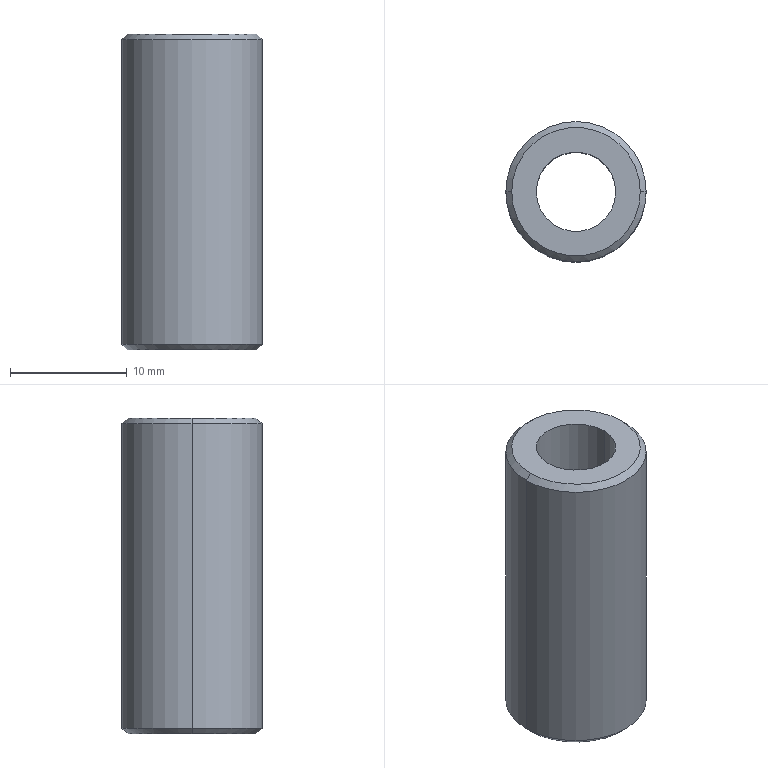Part | STEP file | Screw sleeve QY-1-33 | 1 solid | 10 faces | box 12 x 12 x 27 mm | volume 2064 mm3 | cone 4 | cylinder 4 | plane 2 | commonest cylinder face diameters 6.8 x2 12 x2
STEP:
#1=CARTESIAN_POINT('',(0.,0.,0.));
#2=DIRECTION('',(0.,0.,1.));
#3=DIRECTION('',(1.,0.,0.));
#4=AXIS2_PLACEMENT_3D('',#1,#2,#3);
#5=CARTESIAN_POINT('',(-5.5,0.,0.));
#6=VERTEX_POINT('',#5);
#7=CARTESIAN_POINT('',(5.5,0.,0.));
#8=VERTEX_POINT('',#7);
#9=CARTESIAN_POINT('',(0.,0.,0.));
#10=DIRECTION('',(0.,0.,-1.));
#11=DIRECTION('',(1.,0.,0.));
#12=AXIS2_PLACEMENT_3D('',#9,#10,#11);
#13=CIRCLE('',#12,5.5);
#14=CARTESIAN_POINT('',(0.,0.,0.5));
#15=DIRECTION('',(0.,0.,1.));
#16=DIRECTION('',(1.,0.,0.));
#17=AXIS2_PLACEMENT_3D('',#14,#15,#16);
#18=CONICAL_SURFACE('',#17,6.,0.7854);
#19=CARTESIAN_POINT('',(6.283,-0.5));
#20=DIRECTION('',(-1.,0.));
#21=VECTOR('',#20,1.);
#22=LINE('',#19,#21);
#23=(GEOMETRIC_REPRESENTATION_CONTEXT(2)PARAMETRIC_REPRESENTATION_CONTEXT()REPRESENTATION_CONTEXT('',''));
#24=DEFINITIONAL_REPRESENTATION('',(#22),#23);
#25=PCURVE('',#18,#24);
#26=CARTESIAN_POINT('',(0.,0.,0.));
#27=DIRECTION('',(0.,0.,1.));
#28=DIRECTION('',(1.,0.,0.));
#29=AXIS2_PLACEMENT_3D('',#26,#27,#28);
#30=PLANE('',#29);
#31=CARTESIAN_POINT('',(5.5,0.));
#32=CARTESIAN_POINT('',(5.5,-9.526));
#33=CARTESIAN_POINT('',(-2.75,-4.763));
#34=CARTESIAN_POINT('',(-11.,0.));
#35=CARTESIAN_POINT('',(-2.75,4.763));
#36=CARTESIAN_POINT('',(5.5,9.526));
#37=CARTESIAN_POINT('',(5.5,0.));
#38=(BOUNDED_CURVE()B_SPLINE_CURVE(2,(#31,#32,#33,#34,#35,#36,#37),.UNSPECIFIED.,.T.,.F.)B_SPLINE_CURVE_WITH_KNOTS((1,2,2,2,2,1),(-2.094,0.,2.094,4.189,6.283,8.378),.UNSPECIFIED.)CURVE()GEOMETRIC_REPRESENTATION_ITEM()RATIONAL_B_SPLINE_CURVE((1.,0.5,1.,0.5,1.,0.5,1.))REPRESENTATION_ITEM(''));
#39=(GEOMETRIC_REPRESENTATION_CONTEXT(2)PARAMETRIC_REPRESENTATION_CONTEXT()REPRESENTATION_CONTEXT('',''));
#40=DEFINITIONAL_REPRESENTATION('',(#38),#39);
#41=PCURVE('',#30,#40);
#42=SURFACE_CURVE('',#13,(#25,#41),.PCURVE_S1.);
#43=EDGE_CURVE('',#6,#8,#42,.T.);
#44=ORIENTED_EDGE('',*,*,#43,.F.);
#45=CARTESIAN_POINT('',(-6.,0.,0.5));
#46=VERTEX_POINT('',#45);
#47=CARTESIAN_POINT('',(-6.,0.,0.5));
#48=DIRECTION('',(-0.7071,0.,0.7071));
#49=VECTOR('',#48,1.);
#50=LINE('',#47,#49);
#51=CARTESIAN_POINT('',(3.142,0.));
#52=DIRECTION('',(0.,1.));
#53=VECTOR('',#52,1.);
#54=LINE('',#51,#53);
#55=(GEOMETRIC_REPRESENTATION_CONTEXT(2)PARAMETRIC_REPRESENTATION_CONTEXT()REPRESENTATION_CONTEXT('',''));
#56=DEFINITIONAL_REPRESENTATION('',(#54),#55);
#57=PCURVE('',#18,#56);
#58=CARTESIAN_POINT('',(0.,0.,0.5));
#59=DIRECTION('',(0.,0.,1.));
#60=DIRECTION('',(1.,0.,0.));
#61=AXIS2_PLACEMENT_3D('',#58,#59,#60);
#62=CONICAL_SURFACE('',#61,6.,0.7854);
#63=CARTESIAN_POINT('',(3.142,0.));
#64=DIRECTION('',(0.,1.));
#65=VECTOR('',#64,1.);
#66=LINE('',#63,#65);
#67=(GEOMETRIC_REPRESENTATION_CONTEXT(2)PARAMETRIC_REPRESENTATION_CONTEXT()REPRESENTATION_CONTEXT('',''));
#68=DEFINITIONAL_REPRESENTATION('',(#66),#67);
#69=PCURVE('',#62,#68);
#70=SURFACE_CURVE('',#50,(#57,#69),.PCURVE_S1.);
#71=EDGE_CURVE('',#6,#46,#70,.T.);
#72=ORIENTED_EDGE('',*,*,#71,.T.);
#73=CARTESIAN_POINT('',(6.,0.,0.5));
#74=VERTEX_POINT('',#73);
#75=CARTESIAN_POINT('',(0.,0.,0.5));
#76=DIRECTION('',(0.,0.,1.));
#77=DIRECTION('',(1.,0.,0.));
#78=AXIS2_PLACEMENT_3D('',#75,#76,#77);
#79=CIRCLE('',#78,6.);
#80=CARTESIAN_POINT('',(0.,0.));
#81=DIRECTION('',(1.,0.));
#82=VECTOR('',#81,1.);
#83=LINE('',#80,#82);
#84=(GEOMETRIC_REPRESENTATION_CONTEXT(2)PARAMETRIC_REPRESENTATION_CONTEXT()REPRESENTATION_CONTEXT('',''));
#85=DEFINITIONAL_REPRESENTATION('',(#83),#84);
#86=PCURVE('',#18,#85);
#87=CARTESIAN_POINT('',(0.,0.,27.));
#88=DIRECTION('',(0.,0.,-1.));
#89=DIRECTION('',(-1.,0.,0.));
#90=AXIS2_PLACEMENT_3D('',#87,#88,#89);
#91=CYLINDRICAL_SURFACE('',#90,6.);
#92=CARTESIAN_POINT('',(3.142,26.5));
#93=DIRECTION('',(-1.,0.));
#94=VECTOR('',#93,1.);
#95=LINE('',#92,#94);
#96=(GEOMETRIC_REPRESENTATION_CONTEXT(2)PARAMETRIC_REPRESENTATION_CONTEXT()REPRESENTATION_CONTEXT('',''));
#97=DEFINITIONAL_REPRESENTATION('',(#95),#96);
#98=PCURVE('',#91,#97);
#99=SURFACE_CURVE('',#79,(#86,#98),.PCURVE_S1.);
#100=EDGE_CURVE('',#74,#46,#99,.T.);
#101=ORIENTED_EDGE('',*,*,#100,.F.);
#102=CARTESIAN_POINT('',(6.,0.,0.5));
#103=DIRECTION('',(0.7071,0.,0.7071));
#104=VECTOR('',#103,1.);
#105=LINE('',#102,#104);
#106=CARTESIAN_POINT('',(0.,0.));
#107=DIRECTION('',(0.,1.));
#108=VECTOR('',#107,1.);
#109=LINE('',#106,#108);
#110=(GEOMETRIC_REPRESENTATION_CONTEXT(2)PARAMETRIC_REPRESENTATION_CONTEXT()REPRESENTATION_CONTEXT('',''));
#111=DEFINITIONAL_REPRESENTATION('',(#109),#110);
#112=PCURVE('',#18,#111);
#113=CARTESIAN_POINT('',(6.283,0.));
#114=DIRECTION('',(0.,1.));
#115=VECTOR('',#114,1.);
#116=LINE('',#113,#115);
#117=(GEOMETRIC_REPRESENTATION_CONTEXT(2)PARAMETRIC_REPRESENTATION_CONTEXT()REPRESENTATION_CONTEXT('',''));
#118=DEFINITIONAL_REPRESENTATION('',(#116),#117);
#119=PCURVE('',#62,#118);
#120=SURFACE_CURVE('',#105,(#112,#119),.PCURVE_S1.);
#121=EDGE_CURVE('',#8,#74,#120,.T.);
#122=ORIENTED_EDGE('',*,*,#121,.F.);
#123=EDGE_LOOP('',(#44,#72,#101,#122));
#124=FACE_BOUND('',#123,.T.);
#125=ADVANCED_FACE('',(#124),#18,.T.);
#126=CARTESIAN_POINT('',(5.5,0.,27.));
#127=VERTEX_POINT('',#126);
#128=CARTESIAN_POINT('',(-5.5,0.,27.));
#129=VERTEX_POINT('',#128);
#130=CARTESIAN_POINT('',(0.,0.,27.));
#131=DIRECTION('',(0.,0.,1.));
#132=DIRECTION('',(1.,0.,0.));
#133=AXIS2_PLACEMENT_3D('',#130,#131,#132);
#134=CIRCLE('',#133,5.5);
#135=CARTESIAN_POINT('',(0.,0.,27.));
#136=DIRECTION('',(0.,0.,-1.));
#137=DIRECTION('',(-1.,0.,0.));
#138=AXIS2_PLACEMENT_3D('',#135,#136,#137);
#139=CONICAL_SURFACE('',#138,5.5,0.7854);
#140=CARTESIAN_POINT('',(3.142,0.));
#141=DIRECTION('',(-1.,0.));
#142=VECTOR('',#141,1.);
#143=LINE('',#140,#142);
#144=(GEOMETRIC_REPRESENTATION_CONTEXT(2)PARAMETRIC_REPRESENTATION_CONTEXT()REPRESENTATION_CONTEXT('',''));
#145=DEFINITIONAL_REPRESENTATION('',(#143),#144);
#146=PCURVE('',#139,#145);
#147=CARTESIAN_POINT('',(0.,0.,27.));
#148=DIRECTION('',(0.,0.,1.));
#149=DIRECTION('',(1.,0.,0.));
#150=AXIS2_PLACEMENT_3D('',#147,#148,#149);
#151=PLANE('',#150);
#152=CARTESIAN_POINT('',(0.,0.));
#153=DIRECTION('',(1.,0.));
#154=AXIS2_PLACEMENT_2D('',#152,#153);
#155=CIRCLE('',#154,5.5);
#156=(GEOMETRIC_REPRESENTATION_CONTEXT(2)PARAMETRIC_REPRESENTATION_CONTEXT()REPRESENTATION_CONTEXT('',''));
#157=DEFINITIONAL_REPRESENTATION('',(#155),#156);
#158=PCURVE('',#151,#157);
#159=SURFACE_CURVE('',#134,(#146,#158),.PCURVE_S1.);
#160=EDGE_CURVE('',#127,#129,#159,.T.);
#161=ORIENTED_EDGE('',*,*,#160,.F.);
#162=CARTESIAN_POINT('',(6.,0.,26.5));
#163=VERTEX_POINT('',#162);
#164=CARTESIAN_POINT('',(5.5,0.,27.));
#165=DIRECTION('',(0.7071,0.,-0.7071));
#166=VECTOR('',#165,1.);
#167=LINE('',#164,#166);
#168=CARTESIAN_POINT('',(3.142,0.));
#169=DIRECTION('',(0.,1.));
#170=VECTOR('',#169,1.);
#171=LINE('',#168,#170);
#172=(GEOMETRIC_REPRESENTATION_CONTEXT(2)PARAMETRIC_REPRESENTATION_CONTEXT()REPRESENTATION_CONTEXT('',''));
#173=DEFINITIONAL_REPRESENTATION('',(#171),#172);
#174=PCURVE('',#139,#173);
#175=CARTESIAN_POINT('',(0.,0.,27.));
#176=DIRECTION('',(0.,0.,-1.));
#177=DIRECTION('',(-1.,0.,0.));
#178=AXIS2_PLACEMENT_3D('',#175,#176,#177);
#179=CONICAL_SURFACE('',#178,5.5,0.7854);
#180=CARTESIAN_POINT('',(3.142,0.));
#181=DIRECTION('',(0.,1.));
#182=VECTOR('',#181,1.);
#183=LINE('',#180,#182);
#184=(GEOMETRIC_REPRESENTATION_CONTEXT(2)PARAMETRIC_REPRESENTATION_CONTEXT()REPRESENTATION_CONTEXT('',''));
#185=DEFINITIONAL_REPRESENTATION('',(#183),#184);
#186=PCURVE('',#179,#185);
#187=SURFACE_CURVE('',#167,(#174,#186),.PCURVE_S1.);
#188=EDGE_CURVE('',#127,#163,#187,.T.);
#189=ORIENTED_EDGE('',*,*,#188,.T.);
#190=CARTESIAN_POINT('',(-6.,0.,26.5));
#191=VERTEX_POINT('',#190);
#192=CARTESIAN_POINT('',(0.,0.,26.5));
#193=DIRECTION('',(0.,0.,-1.));
#194=DIRECTION('',(1.,0.,0.));
#195=AXIS2_PLACEMENT_3D('',#192,#193,#194);
#196=CIRCLE('',#195,6.);
#197=CARTESIAN_POINT('',(-3.142,0.5));
#198=DIRECTION('',(1.,0.));
#199=VECTOR('',#198,1.);
#200=LINE('',#197,#199);
#201=(GEOMETRIC_REPRESENTATION_CONTEXT(2)PARAMETRIC_REPRESENTATION_CONTEXT()REPRESENTATION_CONTEXT('',''));
#202=DEFINITIONAL_REPRESENTATION('',(#200),#201);
#203=PCURVE('',#139,#202);
#204=CARTESIAN_POINT('',(-3.142,0.5));
#205=DIRECTION('',(1.,0.));
#206=VECTOR('',#205,1.);
#207=LINE('',#204,#206);
#208=(GEOMETRIC_REPRESENTATION_CONTEXT(2)PARAMETRIC_REPRESENTATION_CONTEXT()REPRESENTATION_CONTEXT('',''));
#209=DEFINITIONAL_REPRESENTATION('',(#207),#208);
#210=PCURVE('',#91,#209);
#211=SURFACE_CURVE('',#196,(#203,#210),.PCURVE_S1.);
#212=EDGE_CURVE('',#191,#163,#211,.T.);
#213=ORIENTED_EDGE('',*,*,#212,.F.);
#214=CARTESIAN_POINT('',(-5.5,0.,27.));
#215=DIRECTION('',(-0.7071,0.,-0.7071));
#216=VECTOR('',#215,1.);
#217=LINE('',#214,#216);
#218=CARTESIAN_POINT('',(0.,0.));
#219=DIRECTION('',(0.,1.));
#220=VECTOR('',#219,1.);
#221=LINE('',#218,#220);
#222=(GEOMETRIC_REPRESENTATION_CONTEXT(2)PARAMETRIC_REPRESENTATION_CONTEXT()REPRESENTATION_CONTEXT('',''));
#223=DEFINITIONAL_REPRESENTATION('',(#221),#222);
#224=PCURVE('',#139,#223);
#225=CARTESIAN_POINT('',(6.283,0.));
#226=DIRECTION('',(0.,1.));
#227=VECTOR('',#226,1.);
#228=LINE('',#225,#227);
#229=(GEOMETRIC_REPRESENTATION_CONTEXT(2)PARAMETRIC_REPRESENTATION_CONTEXT()REPRESENTATION_CONTEXT('',''));
#230=DEFINITIONAL_REPRESENTATION('',(#228),#229);
#231=PCURVE('',#179,#230);
#232=SURFACE_CURVE('',#217,(#224,#231),.PCURVE_S1.);
#233=EDGE_CURVE('',#129,#191,#232,.T.);
#234=ORIENTED_EDGE('',*,*,#233,.F.);
#235=EDGE_LOOP('',(#161,#189,#213,#234));
#236=FACE_BOUND('',#235,.T.);
#237=ADVANCED_FACE('',(#236),#139,.T.);
#238=CARTESIAN_POINT('',(3.4,0.,0.));
#239=VERTEX_POINT('',#238);
#240=CARTESIAN_POINT('',(3.4,0.,27.));
#241=VERTEX_POINT('',#240);
#242=CARTESIAN_POINT('',(3.4,0.,27.));
#243=DIRECTION('',(0.,0.,1.));
#244=VECTOR('',#243,1.);
#245=LINE('',#242,#244);
#246=CARTESIAN_POINT('',(0.,0.,27.));
#247=DIRECTION('',(0.,0.,1.));
#248=DIRECTION('',(1.,0.,0.));
#249=AXIS2_PLACEMENT_3D('',#246,#247,#248);
#250=CYLINDRICAL_SURFACE('',#249,3.4);
#251=CARTESIAN_POINT('',(6.283,0.));
#252=DIRECTION('',(0.,1.));
#253=VECTOR('',#252,1.);
#254=LINE('',#251,#253);
#255=(GEOMETRIC_REPRESENTATION_CONTEXT(2)PARAMETRIC_REPRESENTATION_CONTEXT()REPRESENTATION_CONTEXT('',''));
#256=DEFINITIONAL_REPRESENTATION('',(#254),#255);
#257=PCURVE('',#250,#256);
#258=CARTESIAN_POINT('',(0.,0.,27.));
#259=DIRECTION('',(0.,0.,1.));
#260=DIRECTION('',(1.,0.,0.));
#261=AXIS2_PLACEMENT_3D('',#258,#259,#260);
#262=CYLINDRICAL_SURFACE('',#261,3.4);
#263=CARTESIAN_POINT('',(0.,0.));
#264=DIRECTION('',(0.,1.));
#265=VECTOR('',#264,1.);
#266=LINE('',#263,#265);
#267=(GEOMETRIC_REPRESENTATION_CONTEXT(2)PARAMETRIC_REPRESENTATION_CONTEXT()REPRESENTATION_CONTEXT('',''));
#268=DEFINITIONAL_REPRESENTATION('',(#266),#267);
#269=PCURVE('',#262,#268);
#270=SURFACE_CURVE('',#245,(#257,#269),.PCURVE_S1.);
#271=EDGE_CURVE('',#239,#241,#270,.T.);
#272=ORIENTED_EDGE('',*,*,#271,.T.);
#273=CARTESIAN_POINT('',(-3.4,0.,27.));
#274=VERTEX_POINT('',#273);
#275=CARTESIAN_POINT('',(0.,0.,27.));
#276=DIRECTION('',(0.,0.,1.));
#277=DIRECTION('',(1.,0.,0.));
#278=AXIS2_PLACEMENT_3D('',#275,#276,#277);
#279=CIRCLE('',#278,3.4);
#280=CARTESIAN_POINT('',(0.,0.));
#281=DIRECTION('',(1.,0.));
#282=VECTOR('',#281,1.);
#283=LINE('',#280,#282);
#284=(GEOMETRIC_REPRESENTATION_CONTEXT(2)PARAMETRIC_REPRESENTATION_CONTEXT()REPRESENTATION_CONTEXT('',''));
#285=DEFINITIONAL_REPRESENTATION('',(#283),#284);
#286=PCURVE('',#250,#285);
#287=CARTESIAN_POINT('',(0.,0.));
#288=DIRECTION('',(1.,0.));
#289=AXIS2_PLACEMENT_2D('',#287,#288);
#290=CIRCLE('',#289,3.4);
#291=(GEOMETRIC_REPRESENTATION_CONTEXT(2)PARAMETRIC_REPRESENTATION_CONTEXT()REPRESENTATION_CONTEXT('',''));
#292=DEFINITIONAL_REPRESENTATION('',(#290),#291);
#293=PCURVE('',#151,#292);
#294=SURFACE_CURVE('',#279,(#286,#293),.PCURVE_S1.);
#295=EDGE_CURVE('',#274,#241,#294,.T.);
#296=ORIENTED_EDGE('',*,*,#295,.F.);
#297=CARTESIAN_POINT('',(-3.4,0.,0.));
#298=VERTEX_POINT('',#297);
#299=CARTESIAN_POINT('',(-3.4,0.,27.));
#300=DIRECTION('',(0.,0.,1.));
#301=VECTOR('',#300,1.);
#302=LINE('',#299,#301);
#303=CARTESIAN_POINT('',(3.142,0.));
#304=DIRECTION('',(0.,1.));
#305=VECTOR('',#304,1.);
#306=LINE('',#303,#305);
#307=(GEOMETRIC_REPRESENTATION_CONTEXT(2)PARAMETRIC_REPRESENTATION_CONTEXT()REPRESENTATION_CONTEXT('',''));
#308=DEFINITIONAL_REPRESENTATION('',(#306),#307);
#309=PCURVE('',#250,#308);
#310=CARTESIAN_POINT('',(3.142,0.));
#311=DIRECTION('',(0.,1.));
#312=VECTOR('',#311,1.);
#313=LINE('',#310,#312);
#314=(GEOMETRIC_REPRESENTATION_CONTEXT(2)PARAMETRIC_REPRESENTATION_CONTEXT()REPRESENTATION_CONTEXT('',''));
#315=DEFINITIONAL_REPRESENTATION('',(#313),#314);
#316=PCURVE('',#262,#315);
#317=SURFACE_CURVE('',#302,(#309,#316),.PCURVE_S1.);
#318=EDGE_CURVE('',#298,#274,#317,.T.);
#319=ORIENTED_EDGE('',*,*,#318,.F.);
#320=CARTESIAN_POINT('',(0.,0.,0.));
#321=DIRECTION('',(0.,0.,1.));
#322=DIRECTION('',(1.,0.,0.));
#323=AXIS2_PLACEMENT_3D('',#320,#321,#322);
#324=CIRCLE('',#323,3.4);
#325=CARTESIAN_POINT('',(0.,-27.));
#326=DIRECTION('',(1.,0.));
#327=VECTOR('',#326,1.);
#328=LINE('',#325,#327);
#329=(GEOMETRIC_REPRESENTATION_CONTEXT(2)PARAMETRIC_REPRESENTATION_CONTEXT()REPRESENTATION_CONTEXT('',''));
#330=DEFINITIONAL_REPRESENTATION('',(#328),#329);
#331=PCURVE('',#250,#330);
#332=CARTESIAN_POINT('',(0.,0.));
#333=DIRECTION('',(1.,0.));
#334=AXIS2_PLACEMENT_2D('',#332,#333);
#335=CIRCLE('',#334,3.4);
#336=(GEOMETRIC_REPRESENTATION_CONTEXT(2)PARAMETRIC_REPRESENTATION_CONTEXT()REPRESENTATION_CONTEXT('',''));
#337=DEFINITIONAL_REPRESENTATION('',(#335),#336);
#338=PCURVE('',#30,#337);
#339=SURFACE_CURVE('',#324,(#331,#338),.PCURVE_S1.);
#340=EDGE_CURVE('',#298,#239,#339,.T.);
#341=ORIENTED_EDGE('',*,*,#340,.T.);
#342=EDGE_LOOP('',(#272,#296,#319,#341));
#343=FACE_BOUND('',#342,.F.);
#344=ADVANCED_FACE('',(#343),#250,.F.);
#345=ORIENTED_EDGE('',*,*,#212,.T.);
#346=CARTESIAN_POINT('',(6.,0.,27.));
#347=DIRECTION('',(0.,0.,-1.));
#348=VECTOR('',#347,1.);
#349=LINE('',#346,#348);
#350=CARTESIAN_POINT('',(3.142,0.));
#351=DIRECTION('',(0.,1.));
#352=VECTOR('',#351,1.);
#353=LINE('',#350,#352);
#354=(GEOMETRIC_REPRESENTATION_CONTEXT(2)PARAMETRIC_REPRESENTATION_CONTEXT()REPRESENTATION_CONTEXT('',''));
#355=DEFINITIONAL_REPRESENTATION('',(#353),#354);
#356=PCURVE('',#91,#355);
#357=CARTESIAN_POINT('',(0.,0.,27.));
#358=DIRECTION('',(0.,0.,-1.));
#359=DIRECTION('',(-1.,0.,0.));
#360=AXIS2_PLACEMENT_3D('',#357,#358,#359);
#361=CYLINDRICAL_SURFACE('',#360,6.);
#362=CARTESIAN_POINT('',(3.142,0.));
#363=DIRECTION('',(0.,1.));
#364=VECTOR('',#363,1.);
#365=LINE('',#362,#364);
#366=(GEOMETRIC_REPRESENTATION_CONTEXT(2)PARAMETRIC_REPRESENTATION_CONTEXT()REPRESENTATION_CONTEXT('',''));
#367=DEFINITIONAL_REPRESENTATION('',(#365),#366);
#368=PCURVE('',#361,#367);
#369=SURFACE_CURVE('',#349,(#356,#368),.PCURVE_S1.);
#370=EDGE_CURVE('',#163,#74,#369,.T.);
#371=ORIENTED_EDGE('',*,*,#370,.T.);
#372=ORIENTED_EDGE('',*,*,#100,.T.);
#373=CARTESIAN_POINT('',(-6.,0.,27.));
#374=DIRECTION('',(0.,0.,-1.));
#375=VECTOR('',#374,1.);
#376=LINE('',#373,#375);
#377=CARTESIAN_POINT('',(0.,0.));
#378=DIRECTION('',(0.,1.));
#379=VECTOR('',#378,1.);
#380=LINE('',#377,#379);
#381=(GEOMETRIC_REPRESENTATION_CONTEXT(2)PARAMETRIC_REPRESENTATION_CONTEXT()REPRESENTATION_CONTEXT('',''));
#382=DEFINITIONAL_REPRESENTATION('',(#380),#381);
#383=PCURVE('',#91,#382);
#384=CARTESIAN_POINT('',(6.283,0.));
#385=DIRECTION('',(0.,1.));
#386=VECTOR('',#385,1.);
#387=LINE('',#384,#386);
#388=(GEOMETRIC_REPRESENTATION_CONTEXT(2)PARAMETRIC_REPRESENTATION_CONTEXT()REPRESENTATION_CONTEXT('',''));
#389=DEFINITIONAL_REPRESENTATION('',(#387),#388);
#390=PCURVE('',#361,#389);
#391=SURFACE_CURVE('',#376,(#383,#390),.PCURVE_S1.);
#392=EDGE_CURVE('',#191,#46,#391,.T.);
#393=ORIENTED_EDGE('',*,*,#392,.F.);
#394=EDGE_LOOP('',(#345,#371,#372,#393));
#395=FACE_BOUND('',#394,.T.);
#396=ADVANCED_FACE('',(#395),#91,.T.);
#397=ORIENTED_EDGE('',*,*,#370,.F.);
#398=CARTESIAN_POINT('',(0.,0.,26.5));
#399=DIRECTION('',(0.,0.,-1.));
#400=DIRECTION('',(1.,0.,0.));
#401=AXIS2_PLACEMENT_3D('',#398,#399,#400);
#402=CIRCLE('',#401,6.);
#403=CARTESIAN_POINT('',(3.142,0.5));
#404=DIRECTION('',(1.,0.));
#405=VECTOR('',#404,1.);
#406=LINE('',#403,#405);
#407=(GEOMETRIC_REPRESENTATION_CONTEXT(2)PARAMETRIC_REPRESENTATION_CONTEXT()REPRESENTATION_CONTEXT('',''));
#408=DEFINITIONAL_REPRESENTATION('',(#406),#407);
#409=PCURVE('',#361,#408);
#410=CARTESIAN_POINT('',(3.142,0.5));
#411=DIRECTION('',(1.,0.));
#412=VECTOR('',#411,1.);
#413=LINE('',#410,#412);
#414=(GEOMETRIC_REPRESENTATION_CONTEXT(2)PARAMETRIC_REPRESENTATION_CONTEXT()REPRESENTATION_CONTEXT('',''));
#415=DEFINITIONAL_REPRESENTATION('',(#413),#414);
#416=PCURVE('',#179,#415);
#417=SURFACE_CURVE('',#402,(#409,#416),.PCURVE_S1.);
#418=EDGE_CURVE('',#163,#191,#417,.T.);
#419=ORIENTED_EDGE('',*,*,#418,.T.);
#420=ORIENTED_EDGE('',*,*,#392,.T.);
#421=CARTESIAN_POINT('',(0.,0.,0.5));
#422=DIRECTION('',(0.,0.,1.));
#423=DIRECTION('',(1.,0.,0.));
#424=AXIS2_PLACEMENT_3D('',#421,#422,#423);
#425=CIRCLE('',#424,6.);
#426=CARTESIAN_POINT('',(9.425,26.5));
#427=DIRECTION('',(-1.,0.));
#428=VECTOR('',#427,1.);
#429=LINE('',#426,#428);
#430=(GEOMETRIC_REPRESENTATION_CONTEXT(2)PARAMETRIC_REPRESENTATION_CONTEXT()REPRESENTATION_CONTEXT('',''));
#431=DEFINITIONAL_REPRESENTATION('',(#429),#430);
#432=PCURVE('',#361,#431);
#433=CARTESIAN_POINT('',(0.,0.));
#434=DIRECTION('',(1.,0.));
#435=VECTOR('',#434,1.);
#436=LINE('',#433,#435);
#437=(GEOMETRIC_REPRESENTATION_CONTEXT(2)PARAMETRIC_REPRESENTATION_CONTEXT()REPRESENTATION_CONTEXT('',''));
#438=DEFINITIONAL_REPRESENTATION('',(#436),#437);
#439=PCURVE('',#62,#438);
#440=SURFACE_CURVE('',#425,(#432,#439),.PCURVE_S1.);
#441=EDGE_CURVE('',#46,#74,#440,.T.);
#442=ORIENTED_EDGE('',*,*,#441,.T.);
#443=EDGE_LOOP('',(#397,#419,#420,#442));
#444=FACE_BOUND('',#443,.T.);
#445=ADVANCED_FACE('',(#444),#361,.T.);
#446=CARTESIAN_POINT('',(0.,0.,27.));
#447=DIRECTION('',(0.,0.,1.));
#448=DIRECTION('',(1.,0.,0.));
#449=AXIS2_PLACEMENT_3D('',#446,#447,#448);
#450=CIRCLE('',#449,5.5);
#451=CARTESIAN_POINT('',(0.,0.));
#452=DIRECTION('',(1.,0.));
#453=AXIS2_PLACEMENT_2D('',#451,#452);
#454=CIRCLE('',#453,5.5);
#455=(GEOMETRIC_REPRESENTATION_CONTEXT(2)PARAMETRIC_REPRESENTATION_CONTEXT()REPRESENTATION_CONTEXT('',''));
#456=DEFINITIONAL_REPRESENTATION('',(#454),#455);
#457=PCURVE('',#151,#456);
#458=CARTESIAN_POINT('',(9.425,0.));
#459=DIRECTION('',(-1.,0.));
#460=VECTOR('',#459,1.);
#461=LINE('',#458,#460);
#462=(GEOMETRIC_REPRESENTATION_CONTEXT(2)PARAMETRIC_REPRESENTATION_CONTEXT()REPRESENTATION_CONTEXT('',''));
#463=DEFINITIONAL_REPRESENTATION('',(#461),#462);
#464=PCURVE('',#179,#463);
#465=SURFACE_CURVE('',#450,(#457,#464),.PCURVE_S1.);
#466=EDGE_CURVE('',#129,#127,#465,.T.);
#467=ORIENTED_EDGE('',*,*,#466,.T.);
#468=ORIENTED_EDGE('',*,*,#160,.T.);
#469=EDGE_LOOP('',(#467,#468));
#470=FACE_BOUND('',#469,.T.);
#471=CARTESIAN_POINT('',(0.,0.,27.));
#472=DIRECTION('',(0.,0.,1.));
#473=DIRECTION('',(1.,0.,0.));
#474=AXIS2_PLACEMENT_3D('',#471,#472,#473);
#475=CIRCLE('',#474,3.4);
#476=CARTESIAN_POINT('',(0.,0.));
#477=DIRECTION('',(1.,0.));
#478=AXIS2_PLACEMENT_2D('',#476,#477);
#479=CIRCLE('',#478,3.4);
#480=(GEOMETRIC_REPRESENTATION_CONTEXT(2)PARAMETRIC_REPRESENTATION_CONTEXT()REPRESENTATION_CONTEXT('',''));
#481=DEFINITIONAL_REPRESENTATION('',(#479),#480);
#482=PCURVE('',#151,#481);
#483=CARTESIAN_POINT('',(0.,0.));
#484=DIRECTION('',(1.,0.));
#485=VECTOR('',#484,1.);
#486=LINE('',#483,#485);
#487=(GEOMETRIC_REPRESENTATION_CONTEXT(2)PARAMETRIC_REPRESENTATION_CONTEXT()REPRESENTATION_CONTEXT('',''));
#488=DEFINITIONAL_REPRESENTATION('',(#486),#487);
#489=PCURVE('',#262,#488);
#490=SURFACE_CURVE('',#475,(#482,#489),.PCURVE_S1.);
#491=EDGE_CURVE('',#241,#274,#490,.T.);
#492=ORIENTED_EDGE('',*,*,#491,.F.);
#493=ORIENTED_EDGE('',*,*,#295,.F.);
#494=EDGE_LOOP('',(#492,#493));
#495=FACE_BOUND('',#494,.T.);
#496=ADVANCED_FACE('',(#470,#495),#151,.T.);
#497=CARTESIAN_POINT('',(0.,0.,0.));
#498=DIRECTION('',(0.,0.,-1.));
#499=DIRECTION('',(1.,0.,0.));
#500=AXIS2_PLACEMENT_3D('',#497,#498,#499);
#501=CIRCLE('',#500,5.5);
#502=CARTESIAN_POINT('',(5.5,0.));
#503=CARTESIAN_POINT('',(5.5,-9.526));
#504=CARTESIAN_POINT('',(-2.75,-4.763));
#505=CARTESIAN_POINT('',(-11.,0.));
#506=CARTESIAN_POINT('',(-2.75,4.763));
#507=CARTESIAN_POINT('',(5.5,9.526));
#508=CARTESIAN_POINT('',(5.5,0.));
#509=(BOUNDED_CURVE()B_SPLINE_CURVE(2,(#502,#503,#504,#505,#506,#507,#508),.UNSPECIFIED.,.T.,.F.)B_SPLINE_CURVE_WITH_KNOTS((1,2,2,2,2,1),(-2.094,0.,2.094,4.189,6.283,8.378),.UNSPECIFIED.)CURVE()GEOMETRIC_REPRESENTATION_ITEM()RATIONAL_B_SPLINE_CURVE((1.,0.5,1.,0.5,1.,0.5,1.))REPRESENTATION_ITEM(''));
#510=(GEOMETRIC_REPRESENTATION_CONTEXT(2)PARAMETRIC_REPRESENTATION_CONTEXT()REPRESENTATION_CONTEXT('',''));
#511=DEFINITIONAL_REPRESENTATION('',(#509),#510);
#512=PCURVE('',#30,#511);
#513=CARTESIAN_POINT('',(6.283,-0.5));
#514=DIRECTION('',(-1.,0.));
#515=VECTOR('',#514,1.);
#516=LINE('',#513,#515);
#517=(GEOMETRIC_REPRESENTATION_CONTEXT(2)PARAMETRIC_REPRESENTATION_CONTEXT()REPRESENTATION_CONTEXT('',''));
#518=DEFINITIONAL_REPRESENTATION('',(#516),#517);
#519=PCURVE('',#62,#518);
#520=SURFACE_CURVE('',#501,(#512,#519),.PCURVE_S1.);
#521=EDGE_CURVE('',#8,#6,#520,.T.);
#522=ORIENTED_EDGE('',*,*,#521,.T.);
#523=ORIENTED_EDGE('',*,*,#43,.T.);
#524=EDGE_LOOP('',(#522,#523));
#525=FACE_BOUND('',#524,.T.);
#526=CARTESIAN_POINT('',(0.,0.,0.));
#527=DIRECTION('',(0.,0.,1.));
#528=DIRECTION('',(1.,0.,0.));
#529=AXIS2_PLACEMENT_3D('',#526,#527,#528);
#530=CIRCLE('',#529,3.4);
#531=CARTESIAN_POINT('',(0.,0.));
#532=DIRECTION('',(1.,0.));
#533=AXIS2_PLACEMENT_2D('',#531,#532);
#534=CIRCLE('',#533,3.4);
#535=(GEOMETRIC_REPRESENTATION_CONTEXT(2)PARAMETRIC_REPRESENTATION_CONTEXT()REPRESENTATION_CONTEXT('',''));
#536=DEFINITIONAL_REPRESENTATION('',(#534),#535);
#537=PCURVE('',#30,#536);
#538=CARTESIAN_POINT('',(0.,-27.));
#539=DIRECTION('',(1.,0.));
#540=VECTOR('',#539,1.);
#541=LINE('',#538,#540);
#542=(GEOMETRIC_REPRESENTATION_CONTEXT(2)PARAMETRIC_REPRESENTATION_CONTEXT()REPRESENTATION_CONTEXT('',''));
#543=DEFINITIONAL_REPRESENTATION('',(#541),#542);
#544=PCURVE('',#262,#543);
#545=SURFACE_CURVE('',#530,(#537,#544),.PCURVE_S1.);
#546=EDGE_CURVE('',#239,#298,#545,.T.);
#547=ORIENTED_EDGE('',*,*,#546,.T.);
#548=ORIENTED_EDGE('',*,*,#340,.T.);
#549=EDGE_LOOP('',(#547,#548));
#550=FACE_BOUND('',#549,.T.);
#551=ADVANCED_FACE('',(#525,#550),#30,.F.);
#552=ORIENTED_EDGE('',*,*,#491,.F.);
#553=ORIENTED_EDGE('',*,*,#271,.F.);
#554=ORIENTED_EDGE('',*,*,#546,.T.);
#555=ORIENTED_EDGE('',*,*,#318,.T.);
#556=EDGE_LOOP('',(#552,#553,#554,#555));
#557=FACE_BOUND('',#556,.F.);
#558=ADVANCED_FACE('',(#557),#262,.F.);
#559=ORIENTED_EDGE('',*,*,#188,.F.);
#560=ORIENTED_EDGE('',*,*,#466,.F.);
#561=ORIENTED_EDGE('',*,*,#233,.T.);
#562=ORIENTED_EDGE('',*,*,#418,.F.);
#563=EDGE_LOOP('',(#559,#560,#561,#562));
#564=FACE_BOUND('',#563,.T.);
#565=ADVANCED_FACE('',(#564),#179,.T.);
#566=ORIENTED_EDGE('',*,*,#71,.F.);
#567=ORIENTED_EDGE('',*,*,#521,.F.);
#568=ORIENTED_EDGE('',*,*,#121,.T.);
#569=ORIENTED_EDGE('',*,*,#441,.F.);
#570=EDGE_LOOP('',(#566,#567,#568,#569));
#571=FACE_BOUND('',#570,.T.);
#572=ADVANCED_FACE('',(#571),#62,.T.);
#573=CLOSED_SHELL('',(#125,#237,#344,#396,#445,#496,#551,#558,#565,#572));
#574=MANIFOLD_SOLID_BREP('',#573);
#575=(LENGTH_UNIT()NAMED_UNIT(*)SI_UNIT(.MILLI.,.METRE.));
#576=UNCERTAINTY_MEASURE_WITH_UNIT(LENGTH_MEASURE(0.0000001),#575,'','');
#577=(NAMED_UNIT(*)PLANE_ANGLE_UNIT()SI_UNIT($,.RADIAN.));
#578=(NAMED_UNIT(*)SI_UNIT($,.STERADIAN.)SOLID_ANGLE_UNIT());
#579=(GEOMETRIC_REPRESENTATION_CONTEXT(3)GLOBAL_UNCERTAINTY_ASSIGNED_CONTEXT((#576))GLOBAL_UNIT_ASSIGNED_CONTEXT((#575,#577,#578))REPRESENTATION_CONTEXT('',''));
#580=ADVANCED_BREP_SHAPE_REPRESENTATION('',(#4,#574),#579);